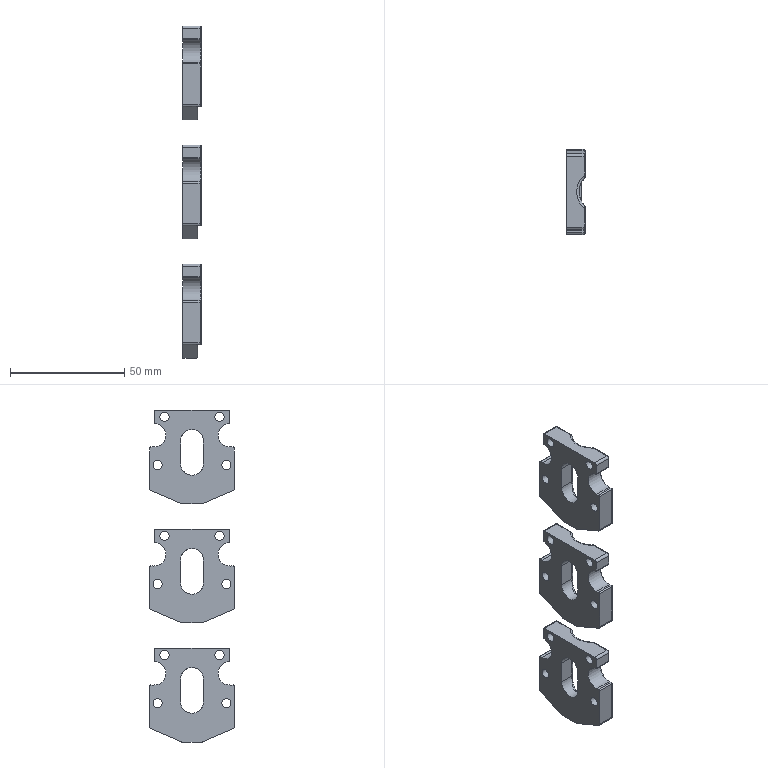CAM job | NX | 3+2 milling, drilling | part box 8 x 37 x 145 mm | stock box 10 x 40 x 150 mm
Tools:
number,name,description,diameter,corner_radius,flute_length,length,flutes
3,D3,平底铣刀-粗,3.0,0.0,20.0,75.0,2
6,D6,平底铣刀-粗,6.0,0.0,25.0,75.0,2
9,D10,平底铣刀-粗,10.0,0.0,35.0,75.0,2
7,D6-J,平底铣刀-精,6.0,0.0,25.0,75.0,2
10,D10-J,平底铣刀-精,10.0,0.0,35.0,75.0,2
1,D80R0.8飞刀,圆鼻刀-粗,80.0,0.8,50.0,75.0,2
1,D80R0.8飞刀-J,圆鼻刀-精,80.0,0.8,50.0,75.0,2
2,D6倒角刀,倒角刀,6.0,0.0,3.0,25.0,2
18,R1.5,圆球刀,3.0,1.5,10.0,50.0,2
17,ZT4,钻头,4.0,0.0,35.0,50.0,2
Operations:
program,operation,operation_type,tool,method,geometry_group,spindle_rpm,surface_speed,feed_per_tooth,feed_cut,feed_plunge,cut_length_mm,path_length_mm,cut_time_min,machine_time_min
B,底壁铣飞面一刀开粗_COPY,VolumeBased25DMillingOperation,D80R0.8飞刀,分层开粗-切深K-步距G,W-B,2800.0,703.696,0.5357,3000.0,100.0,1012.776,1794.734,0.3376,0.4158
B,底壁铣飞面一刀精光_COPY,VolumeBased25DMillingOperation,D80R0.8飞刀-J,侧刃精光-切深K-步距G,W-B,4000.0,1005.28,0.125,1000.0,100.0,252.998,288.998,0.253,0.2566
B,平面去毛刺6X45L_COPY,SurfaceContour,D6倒角刀,爬面_倒角-切深0-步距G,W-B,6500.0,122.519,0.1154,1500.0,100.0,768.292,1580.57,0.5122,0.5934
A,顶面,FaceMilling,D80R0.8飞刀,侧刃精光-切深K-步距G,W-A,5000.0,1256.637,0.1,1000.0,100.0,239.0,275.0,0.239,0.2426
A,外形粗_2,VolumeBased25DMillingOperation,D10,METHOD,W-A,8000.0,251.327,0.3125,5000.0,80.0,6787.998,7033.602,1.358,1.382
A,型腔铣开粗-中_COPY,CavityMilling,D6,分层开粗-切深K-步距G,W-A,8000.0,150.796,0.125,2000.0,100.0,25502.491,27572.872,12.751,13.029
A,型腔铣分层二粗-中_COPY,CavityMilling,D3,分层开粗-切深K-步距G,W-A,8000.0,75.398,0.0063,100.0,100.0,2660.836,4374.48,26.608,26.82
A,打点-深0.8,Operation,D6倒角刀,NONE,W-A,8000.0,150.796,0.0312,500.0,90.0,21.6,369.141,0.0432,0.078
A,通孔-精孔4.0预钻,Operation,ZT4,NONE,W-A,3000.0,36.757,0.0417,250.0,90.0,158.421,642.782,0.6337,0.6821
A,钻倒角_1,Operation,D6倒角刀,METHOD,W-A,8000.0,150.796,0.0312,500.0,0.0,63.6,476.949,0.1272,0.1685
A,曲面D4R2,SurfaceContour,R1.5,METHOD,W-A,7000.0,65.973,0.25,3500.0,100.0,29493.875,30227.581,8.427,8.5
A,曲面D4R2_COPY,SurfaceContour,R1.5,METHOD,W-A,7000.0,65.973,0.25,3500.0,100.0,18658.537,19659.416,5.331,5.431
A,等高精光往复爬面_COPY,ZLevelMilling,R1.5,等高爬面-切深K-步距G,W-A,7000.0,65.973,0.25,3500.0,100.0,3483.744,4086.191,0.9954,1.056
A,底精_1,VolumeBased25DMillingOperation,D6-J,METHOD,W-A,6000.0,113.0,0.2083,1200.0,100.0,234.7,478.651,0.1956,0.22
A,底侧精_3,VolumeBased25DMillingOperation,D6-J,METHOD,W-A,6000.0,113.0,0.0667,800.0,100.0,140.711,526.863,0.1759,0.2145
A,底壁铣精光侧面-中_COPY,VolumeBased25DMillingOperation,D6-J,侧刃精光-切深K-步距G,W-A,6000.0,113.097,0.0667,800.0,100.0,237.968,444.347,0.2975,0.3181
A,外形半精_2,VolumeBased25DMillingOperation,D10-J,METHOD,W-A,8000.0,251.327,0.0625,1000.0,100.0,579.412,778.104,0.5794,0.5993